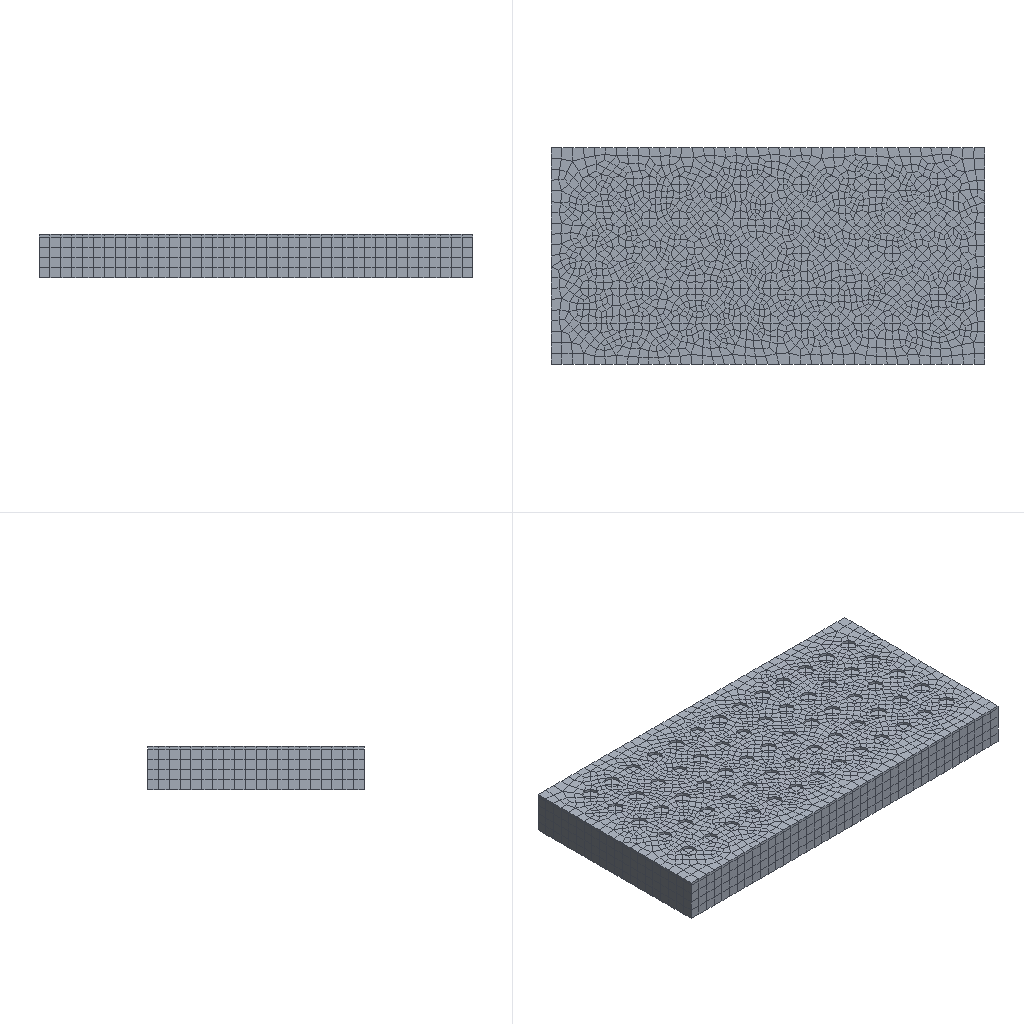Simulation study | abaqus
Set-up summary:
category,name,step,type,value,unit,region
solver,abaqus
solver,version,,,Abaqus/Standard 3DEXPERIENCE R2017x
units,not stated in the deck,,not stated
analysis,deck,,thermal,thermal
load_step,Step-1,Step-1,thermal
load_step,requested,,,1
mesh,nodes,,,12433
mesh,elements,,,9850
element_type,DC3D8,,solid,9850
load,load commands in deck,,count,2
bc,support commands in deck,,count,1
material,MATERIAL-1,,in results
check,setup vs results,,match,"per instance, exact: element labels, types and connectivity; labels of the nodes the elements use; coordinates of those nodes at SINGLE_PRECISION in 1 of 1 instance(s)"
Abaqus input file, long lists of numbers shortened:
*Heading
** Job name: Job-1 Model name: Model-1
** Generated by: Abaqus/CAE 2017
*Preprint, echo=NO, model=NO, history=NO, contact=NO
**
** PARTS
**
*Part, name=work
*Node
      1,   2.016,  -1.976,         1.87
      2,   4.816,  -1.976,         1.87
** (12431 more lines like these left out)
*Element, type=DC3D8
   1, 1700,  595,  594, 2327, 3078,  716,  717, 3705
   2, 1700, 2327, 2150, 1829, 3078, 3705, 3528, 3207
** (9848 more lines like these left out)
*Nset, nset=Set-1, generate
     1,  12433,      1
*Elset, elset=Set-1, generate
    1,  9850,     1
** Section: Section-1
*Solid Section, elset=Set-1, material=Material-1
,
*End Part
**
**
** ASSEMBLY
**
*Assembly, name=Assembly
**
*Instance, name=work-1, part=work
*End Instance
**
*Node
      1,   1.733,  -1.693,           2.
*Node
      2,           0.,  -1.693,           2.
*Node
      3,   1.733,  -3.293,           2.
*Node
      4,           0.,   -3.293,           2.
*Node
      5,           0.,  -4.893,           2.
*Node
      6,           0.,  -6.493,           2.
*Node
      7,           0.,  -8.093,           2.
*Node
      8,          20.,   -3.293,           2.
*Node
      9,          20.,  -6.493,           2.
*Nset, nset=Set-1, instance=work-1, generate
     1,  12433,      1
*Elset, elset=Set-1, instance=work-1, generate
    1,  9850,     1
*Elset, elset=_Surf-1_S6, internal, instance=work-1
   12,   14,   18,   25,   38,   42,   53,   76,   77,   80,   83,   86,   95,   98,  103,  115
  122,  128,  129,  133,  136,  138,  146,  149,  154,  165,  174,  177,  181,  197,  206,  220
** (18 more lines like these left out)
*Elset, elset=_Surf-1_S4, internal, instance=work-1
    1,    7,   11,   19,   26,   30,   36,   44,   51,   68,   69,   70,   82,   94,  101,  123
  130,  142,  144,  150,  155,  163,  170,  194,  200,  204,  211,  215,  221,  228,  230,  243
** (22 more lines like these left out)
*Elset, elset=_Surf-1_S3, internal, instance=work-1
    5,   23,   43,   48,   54,   59,   61,   73,   87,   88,   99,  117,  120,  124,  125,  132
  153,  159,  160,  161,  169,  178,  182,  186,  188,  190,  192,  198,  201,  209,  234,  252
** (14 more lines like these left out)
*Elset, elset=_Surf-1_S5, internal, instance=work-1
    6,   16,   17,   27,   35,   40,   49,   74,   78,   96,  104,  108,  112,  135,  140,  145
  173,  208,  218,  224,  240,  249,  256,  271,  293,  300,  305,  310,  313,  324,  329,  346
** (10 more lines like these left out)
*Elset, elset=_Surf-1_S1, internal, instance=work-1, generate
 1763,  2022,     1
*Elset, elset=_Surf-1_S2, internal, instance=work-1
    1,    2,    3,    4,    5,    6,    7,    8,    9,   10,   11,   12,   13,   14,   15,   16
   17,   18,   19,   20,   21,   22,   23,   24,   25,   26,   27,   28,   29,   30,   31,   32
** (235 more lines like these left out)
*Surface, type=ELEMENT, name=Surf-1
_Surf-1_S6, S6
_Surf-1_S4, S4
_Surf-1_S2, S2
_Surf-1_S3, S3
_Surf-1_S5, S5
_Surf-1_S1, S1
*End Assembly
**
** MATERIALS
**
*Material, name=Material-1
*Conductivity
52.,
*Density
 7.8e-09,
*Elastic
210000., 0.3
*Expansion
 1.5e-05,
*Plastic, hardening=JOHNSON COOK
792.,  510., 0.014,  0.04, 2000.,   20.
*Specific Heat
 5e+08,
**
** PHYSICAL CONSTANTS
**
*Physical Constants, absolute zero=-273., stefan boltzmann=5.67e-08
** ----------------------------------------------------------------
**
** STEP: Step-1
**
*Step, name=Step-1, nlgeom=NO, inc=10000
*Heat Transfer, end=PERIOD, deltmx=100000., mxdem=1.
1., 100., 0.001, 100.,
**
** LOADS
**
** Name: Load-1   Type: Body heat flux
*Dflux
Set-1, BFNU, 1.
**
** INTERACTIONS
**
** Interaction: Int-1
*Sradiate
Surf-1, R, 20., 0.1
**
** OUTPUT REQUESTS
**
*Restart, write, frequency=0
**
** FIELD OUTPUT: F-Output-1
**
*Output, field, variable=PRESELECT
*Output, history, frequency=0
*End Step
Results summary:
result,step,,partial,increments=0 time=0.0/100.0
result,analysis,,,"heat transfer, deltamx"
result,last_loadstep,,,1
result,primary field,,,NT11